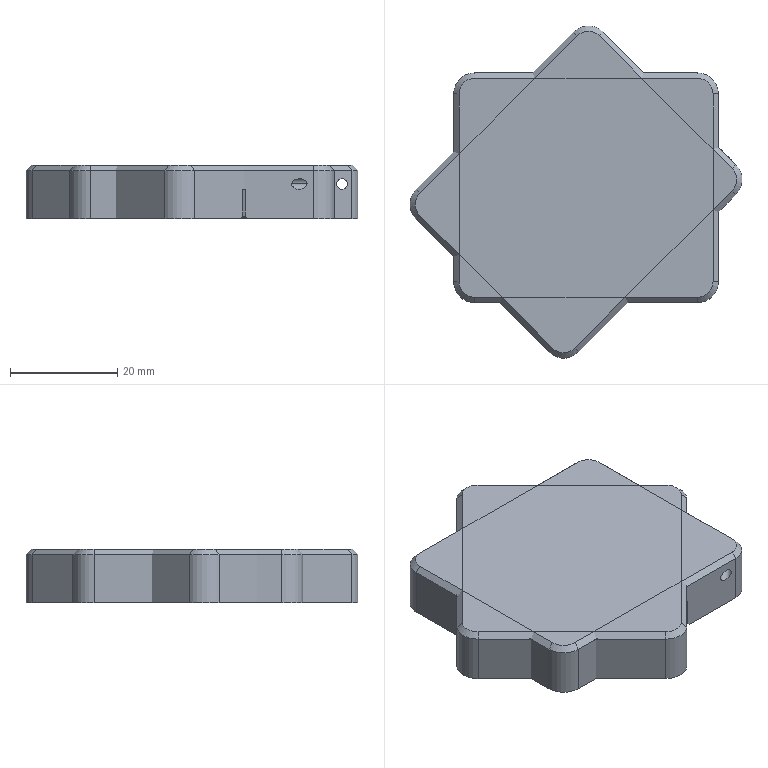NC program | NX | posted with a generic post | part box 61.954 x 61.954 x 10 mm
Whole program:
N10 G17 G21 G94 G90
(PLANAR_MILL_4 , TOOL : D8倒角刀)
N12 T05 M6
N14 G54
N16 G17 G0 G90 X-28.795 Y63.661 B0. C0. S100 M3
N18 G43 Z30. H5
N20 Z3.
N22 G94 G1 Z0. F1000.
N24 X-23.138 Y58.004
N26 X60.654 Y-25.788
N28 X66.311 Y-31.445
N30 Z3.
N32 G0 Z30.
N34 M5
N36 M2